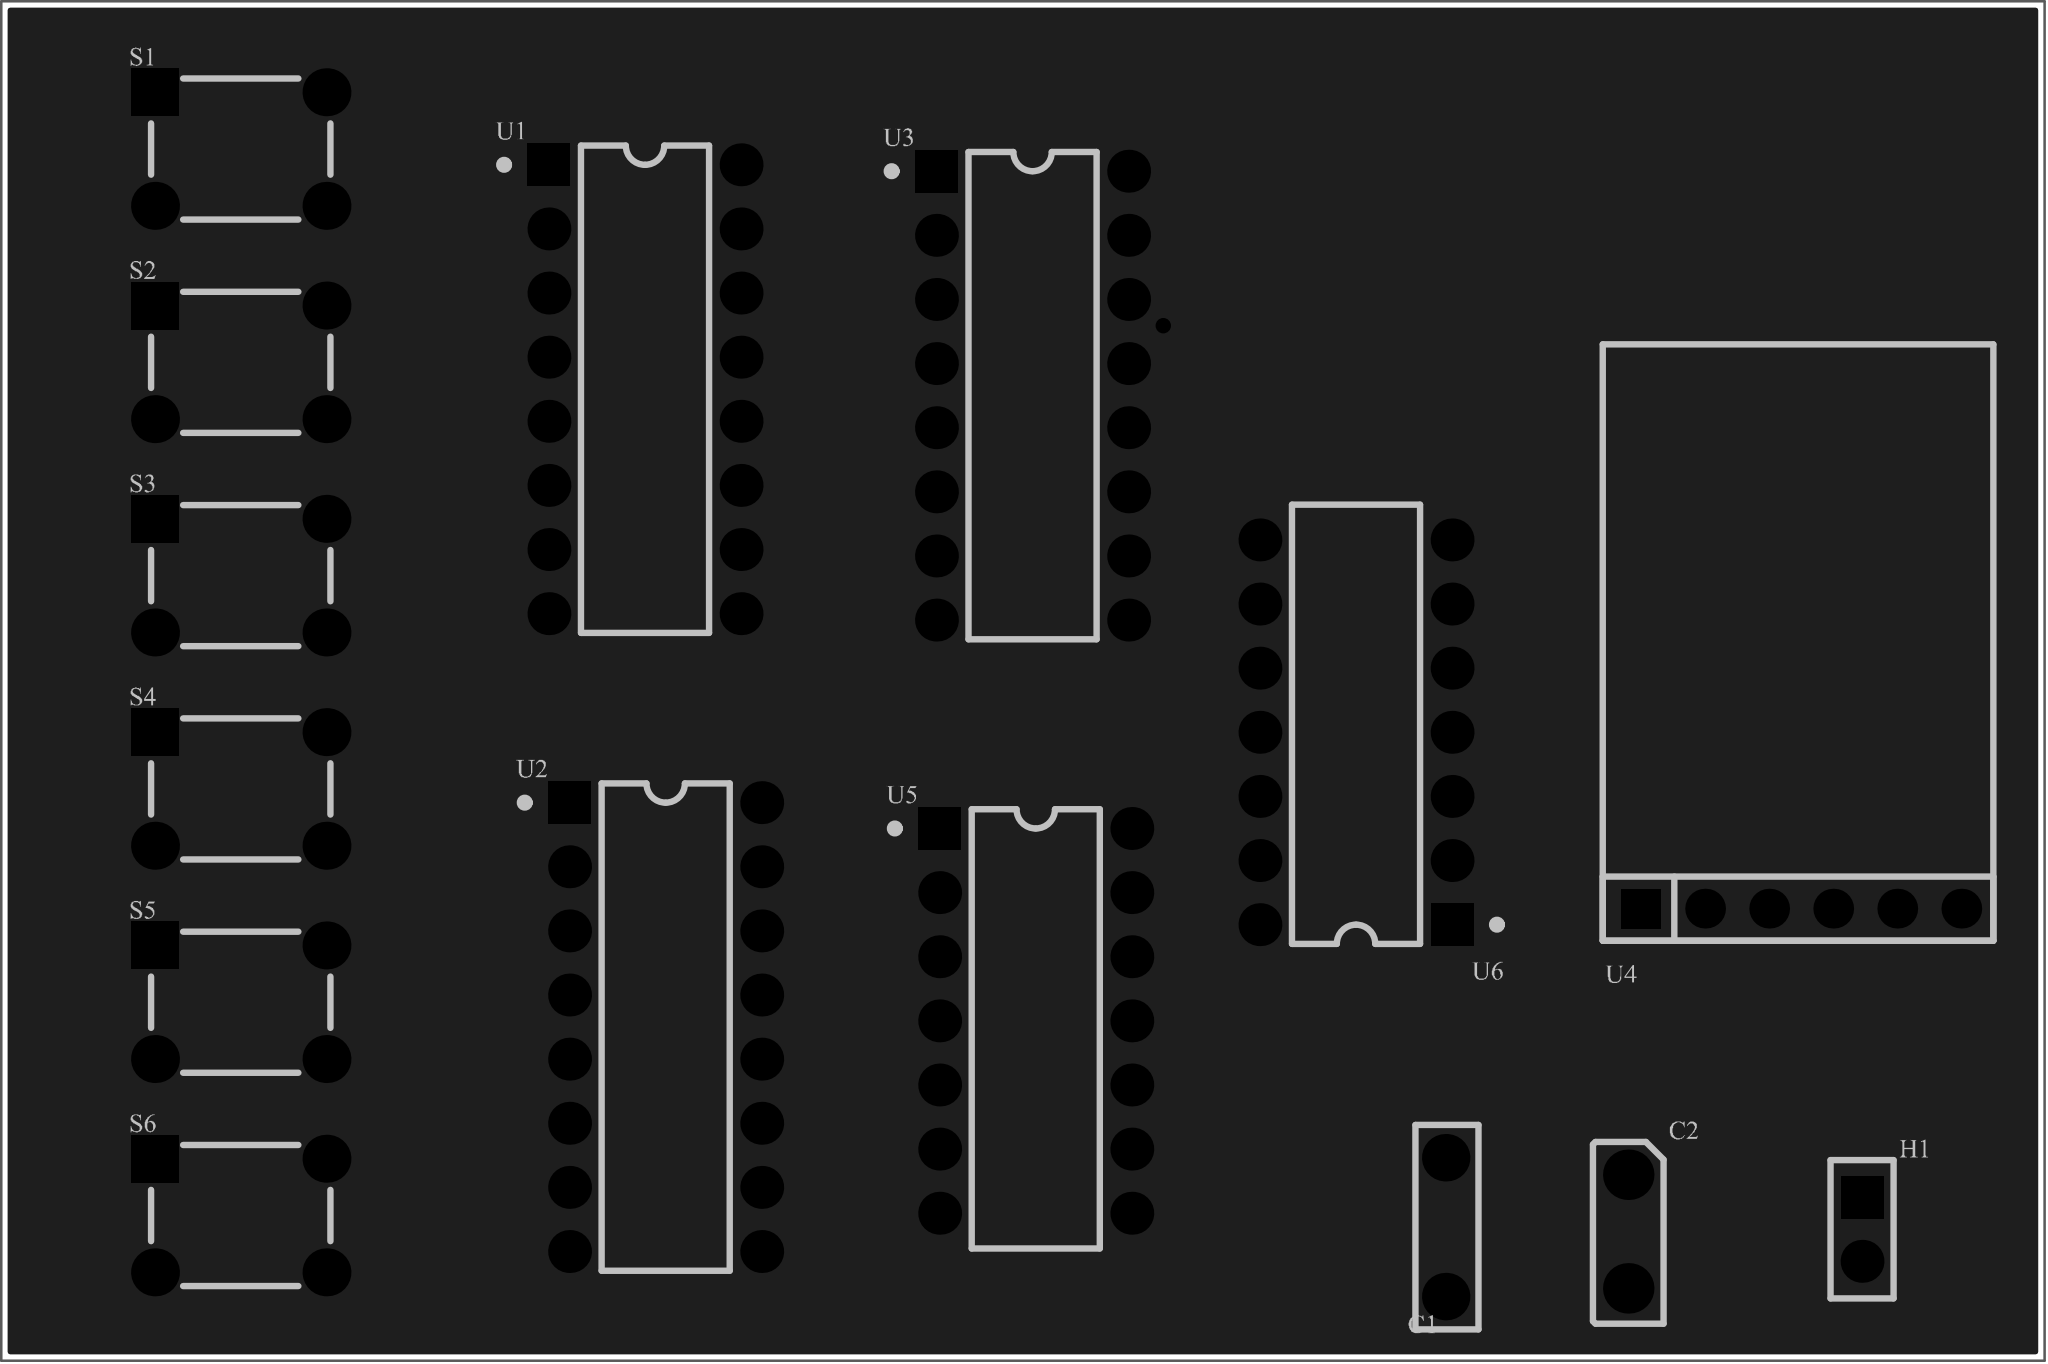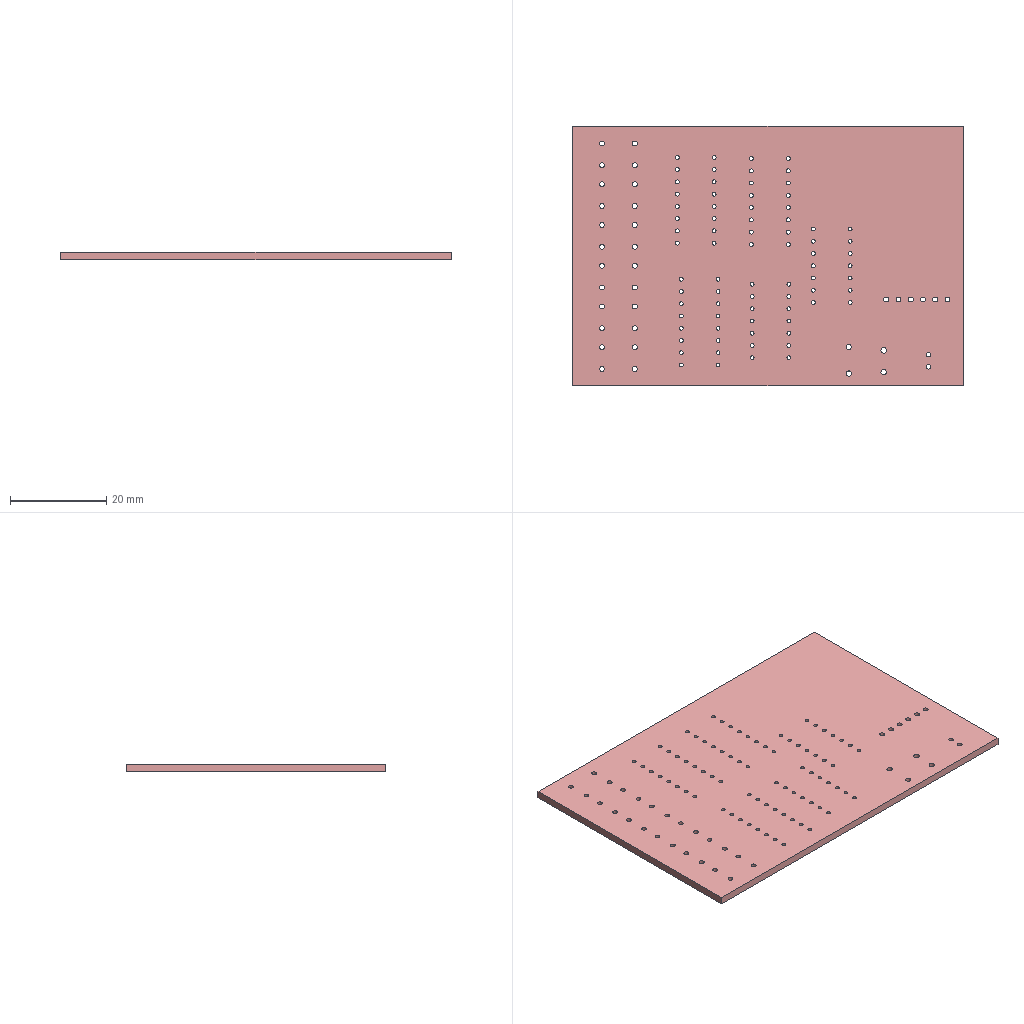Circuit board layout | Altium Designer | box 81 x 53.8 x 1.6 mm
Layer stack:
# Altium Designer layer stack of  (unit mm; dielectric type: 0 none, 1 core, 2 prepreg, 3 surface material)
index,name,kind,layer,copper_thickness_mm,dielectric_type,dielectric_thickness_mm,dielectric_material,dielectric_constant
0,Top Paste Mask Layer,other,,,,,,
1,Top Silkscreen Layer,other,,,,,,
2,Top Solder Mask Layer,dielectric,,,3,0.01,,3.3
3,Top Layer,copper,Top Layer,0.035,,,,
4,Dielectric1,dielectric,,,3,1.51,FR4,4.5
5,Bottom Layer,copper,Bottom Layer,0.035,,,,
6,Bottom Solder Mask Layer,dielectric,,,3,0.01,,3.3
7,Bottom Silkscreen Layer,other,,,,,,
8,Bottom Paste Mask Layer,other,,,,,,
# drill layer pairs: low layer,high layer
drill_pair,Top Layer,Bottom Layer
Part placement:
Designator,Comment,Layer,Footprint,Center-X(mm),Center-Y(mm),Rotation
C1,0.1uF,TopLayer,CAP,143.256,90.761,90
C2,10uF,TopLayer,CAP_POL,150.495,90.587,270
S1,KEY,TopLayer,KEY-4,95.475,133.466,0
S2,KEY,TopLayer,KEY-4,95.475,125.017,0
S3,KEY,TopLayer,KEY-4,95.475,116.568,0
S4,KEY,TopLayer,KEY-4,95.475,108.12,0
S5,KEY,TopLayer,KEY-4,95.475,99.671,0
S6,KEY,TopLayer,KEY-4,95.475,91.222,0
U1,74LS75D,TopLayer,74LS75D,111.506,123.952,0
U2,74LS75D,TopLayer,74LS75D,112.324,98.686,0
U3,74LS148D,TopLayer,74LS148D,126.873,123.698,0
U4,DCD_HEX,TopLayer,SMG,157.353,103.378,0
U5,74LS32,TopLayer,74LS32,127,98.933,0
U6,74LS04,TopLayer,74LS04,139.7,110.363,180
H1,,TopLayer,HDR-TH_2P-P2.54-V-F,159.766,90.678,270
Pad and via stacks:
# Altium Designer via and pad stacks of  (unit mm). Each distinct definition once, with the count of objects using it.
# via: kind,start_layer,end_layer,hole_mm,diameter_mm,mode(0 simple;1 top-mid-bottom;2 full stack),diameter_per_layer,count,example_net
# pad: kind,layer,hole_mm,hole_type(0 round;1 square;2 slot),plating,top_size,top_shape(1 round;2 rect;3 octagon;9 rounded rect),mid_size,bottom_size,mode,footprint,size_per_layer,count,example
pad,Multi-Layer,1.1,0,plated,1.88x1.88,1,1.88x1.88,1.88x1.88,0,CAP,,2,C1.2
pad,Multi-Layer,1.2,0,plated,2x2,1,2x2,2x2,0,CAP POL,,2,C2.2
pad,Multi-Layer,1,0,plated,1.9x1.9,1,1.9x1.9,1.9x1.9,0,KEY-4,,18,S1.4
pad,Multi-Layer,1,0,plated,1.9x1.9,2,1.9x1.9,1.9x1.9,0,KEY-4,,6,S1.1
pad,Multi-Layer,0.8,0,plated,1.7x1.7,1,1.7x1.7,1.7x1.7,0,74LS75D,,30,U1.9
pad,Multi-Layer,0.8,0,plated,1.7x1.7,2,1.7x1.7,1.7x1.7,0,74LS75D,,2,U1.1
pad,Multi-Layer,0.8,0,plated,1.7x1.7,1,1.7x1.7,1.7x1.7,0,74LS148D,,15,U3.9
pad,Multi-Layer,0.8,0,plated,1.7x1.7,2,1.7x1.7,1.7x1.7,0,74LS148D,,1,U3.1
pad,Multi-Layer,1.02,0,plated,1.575x1.575,2,1.575x1.575,1.575x1.575,0,SMG,,1,U4.1
pad,Multi-Layer,1.02,0,plated,1.575x1.575,1,1.575x1.575,1.575x1.575,0,SMG,,5,U4.2
pad,Multi-Layer,0.8,0,plated,1.7x1.7,1,1.7x1.7,1.7x1.7,0,74LS32,,13,U5.9
pad,Multi-Layer,0.8,0,plated,1.7x1.7,2,1.7x1.7,1.7x1.7,0,74LS32,,1,U5.1
pad,Multi-Layer,0.8,0,plated,1.7x1.7,1,1.7x1.7,1.7x1.7,0,74LS04,,13,U6.14
pad,Multi-Layer,0.8,0,plated,1.7x1.7,2,1.7x1.7,1.7x1.7,0,74LS04,,1,U6.1
pad,Multi-Layer,1,0,plated,1.7x1.7,2,1.7x1.7,1.7x1.7,0,HDR-TH_2P-P2.54-V-F,,1,H1.1
pad,Multi-Layer,1,0,plated,1.7x1.7,1,1.7x1.7,1.7x1.7,0,HDR-TH_2P-P2.54-V-F,,1,H1.2
via,Top Layer,Bottom Layer,0.3048,0.61,0,,1,GND
Copper pours:
name,layer,net,type(0 solid;1 hatched;2 none)
Top Layer-GND,Top Layer,GND,0
Bottom Layer-GND,Bottom Layer,GND,0
Design rules, without the lines most boards share:
# Altium Designer design rules of  (exported by Altium Designer, unit mm)
# columns: name | kind | enabled | priority | scope1 | scope2 | descriptor | typed fields (field=value)
creepage | 65 | enabled | 1 | All | All | Creepage Distance Constraint =(0mil) (All),(All) |